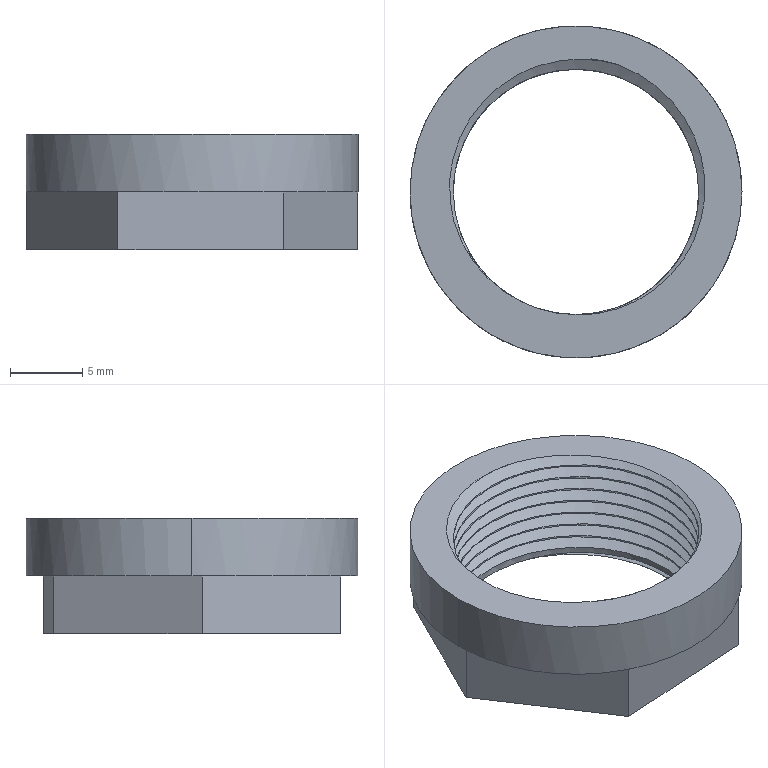Part | SolidWorks | features MBimport 1 | 1 solid | 36 faces | box 23 x 23 x 8 mm | volume 1078 mm3 | cylinder 20 | plane 14 | spline 2 | commonest cylinder face diameters 17 x18 23 x2